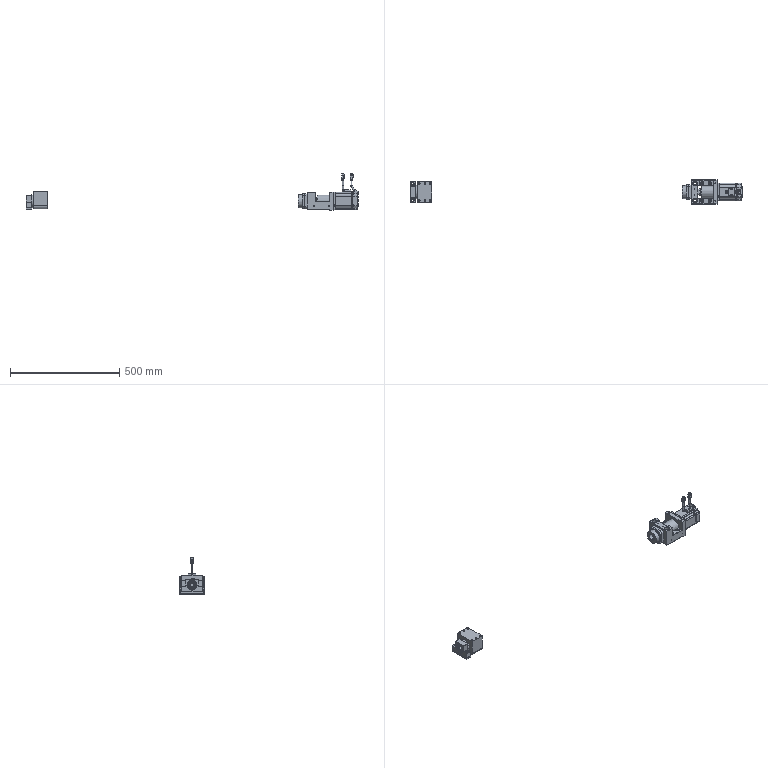Part | NX | 16 solids | 1029 faces | box 1518 x 110 x 167.8 mm | volume 1847627 mm3 | plane 670 | cylinder 283 | cone 51 | spline 25 | commonest cylinder face diameters 8 x44 15 x28 0.6 x18 7 x15 6 x14 11 x12